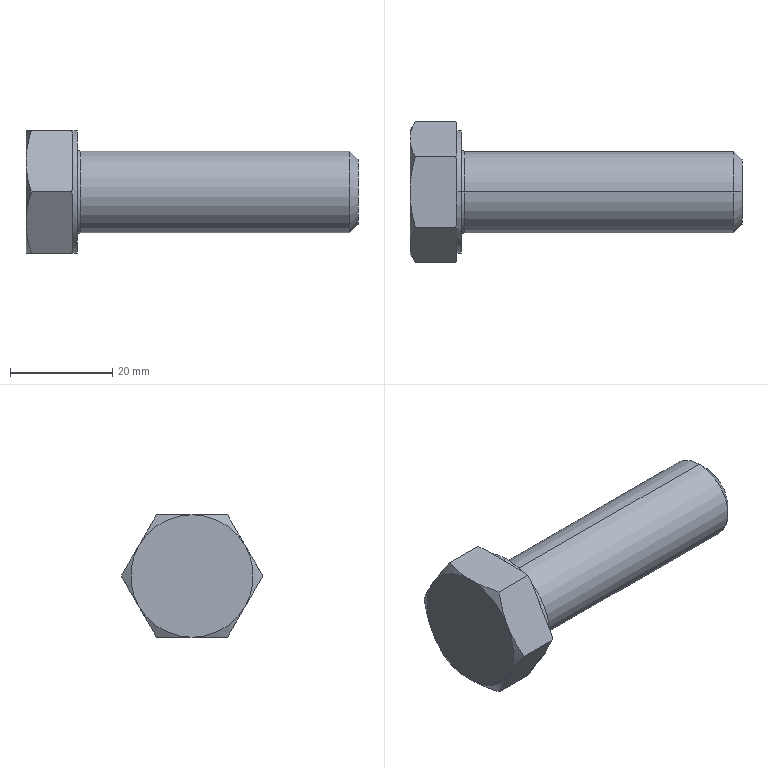Part | STEP file | 1 solid | 35 faces | box 65 x 27.713 x 24 mm | volume 15938 mm3 | plane 15 | cone 14 | cylinder 4 | spline 2 | commonest cylinder face diameters 16 x2 24 x2